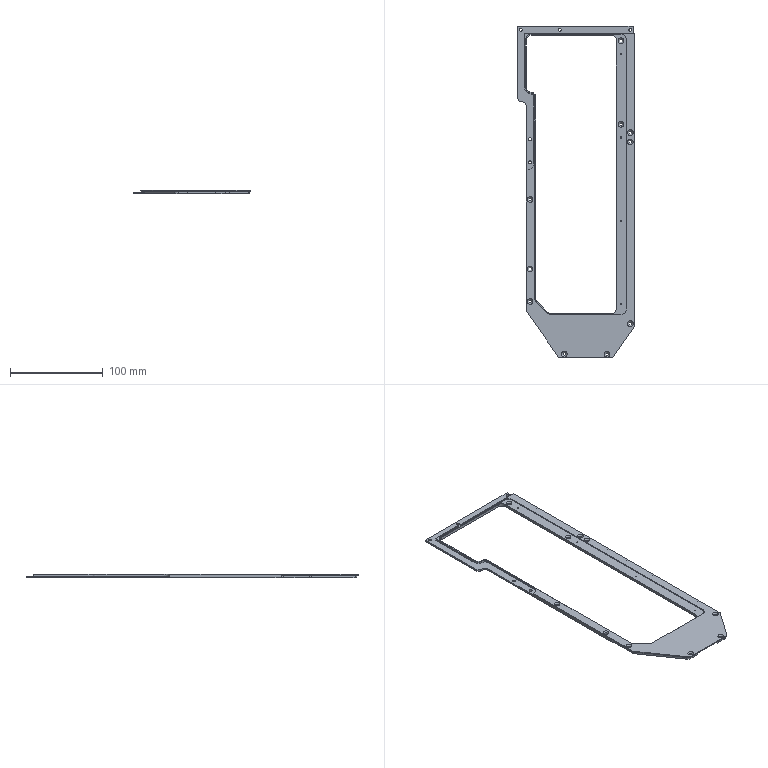CAM job | NX | 3-axis milling, drilling | part box 127 x 358 x 4 mm | stock box 134 x 366 x 4 mm
Tools:
number,name,description,diameter,corner_radius,flute_length,length,flutes
4,D6-18-D6-50-3T-ROUGH,D6-18-D6-50-3T-粗,6.0,0.0,18.0,50.0,2
5,D6-18-D6-50-3T-FINISH,D6-18-D6-50-3T,6.0,0.0,18.0,50.0,3
7,DRILL_D1.84-11-D3-40,钻刀D1.84-11-D3-40,1.84,0.0,11.0,12.0,2
3,DRILL_D3.2-42-71,钻刀D3.2-42-71,3.2,0.0,42.0,71.0,2
0,DRILL_D4.3-54-83,钻刀D4.3-54-83,4.3,0.0,54.0,83.0,2
2,DRILL_D5.3-62-92,钻刀D5.3-62-92,5.3,0.0,62.0,92.0,2
8,FORMTAP_M2-12-D3-39,挤压M2-12-D3-39,2.0,0.0,12.5,14.5,2
0,UPPERROW_M5-22-D5.5-60,上排M5-22-D5.5-60,5.0,0.0,22.0,25.0,2
6,CHAMFER_D3-90DEG,倒角D3-90度,3.0,0.0,5.0,50.0,2
1,CHAMFER_D8-90DEG,倒角D8-90度,8.0,0.0,8.0,60.0,2
Operations:
program,operation,operation_type,tool,method,geometry_group,spindle_rpm,surface_speed,feed_per_tooth,feed_cut,feed_plunge,cut_length_mm,path_length_mm,cut_time_min,machine_time_min
A1,SPOT_DRILL,Operation,CHAMFER_D8-90DEG,METHOD,WORKPIECE,2500.0,62.0,0.05,250.0,0.0,78.4,853.725,0.3136,0.3911
A1,SPOT_DRILL_COPY,Operation,DRILL_D5.3-62-92,METHOD,WORKPIECE,3000.0,0.0,0.0,200.0,0.0,133.0,962.925,0.665,0.748
A2,SPOT_DRILL_1,Operation,CHAMFER_D8-90DEG,METHOD,WORKPIECE,2500.0,62.0,0.05,250.0,0.0,69.0,907.539,0.276,0.3599
A2,SPOT_DRILL_1_COPY,Operation,DRILL_D3.2-42-71,METHOD,WORKPIECE,3000.0,0.0,0.0,200.0,0.0,135.0,1039.539,0.675,0.7655
A2,PLANAR_MILL_9,PlanarMilling,D6-18-D6-50-3T-ROUGH,METHOD,A-G54,3500.0,65.0,0.2143,1500.0,100.0,293.379,600.371,0.1956,0.2263
A2,FLOOR_FACING,VolumeBased25DMillingOperation,D6-18-D6-50-3T-ROUGH,METHOD,A-G54,3500.0,65.0,0.2143,1500.0,100.0,1620.379,1796.036,1.08,1.098
A2,PLANAR_MILL,PlanarMilling,D6-18-D6-50-3T-ROUGH,METHOD,A-G54,3500.0,65.0,0.2143,1500.0,100.0,168.708,207.508,0.1125,0.1164
A2,PLANAR_MILL_1_COPY_1,PlanarMilling,D6-18-D6-50-3T-ROUGH,METHOD,A-G54,3500.0,65.0,0.2143,1500.0,100.0,4139.758,4868.484,2.76,2.833
A2,PLANAR_MILL_1_COPY_1_COPY,PlanarMilling,D6-18-D6-50-3T-ROUGH,METHOD,A-G54,3500.0,65.0,0.2143,1500.0,100.0,715.0,1458.8,0.4767,0.551
A2,PLANAR_MILL_1,PlanarMilling,D6-18-D6-50-3T-ROUGH,METHOD,A-G54,3500.0,65.0,0.2143,1500.0,100.0,1614.092,2336.95,1.076,1.148
A2,PLANAR_MILL_9_COPY,PlanarMilling,D6-18-D6-50-3T-FINISH,METHOD,A-G54,3500.0,65.0,0.1429,500.0,100.0,80.291,394.36,0.1606,0.192
A2,FLOOR_FACING_COPY,VolumeBased25DMillingOperation,D6-18-D6-50-3T-FINISH,METHOD,A-G54,3500.0,65.0,0.0762,800.0,100.0,542.755,581.755,0.6784,0.6823
A2,PLANAR_MILL_COPY,PlanarMilling,D6-18-D6-50-3T-FINISH,METHOD,A-G54,3500.0,65.0,0.0762,800.0,100.0,169.908,208.908,0.2124,0.2163
A2,PLANAR_MILL_1_COPY_1_COPY_1,PlanarMilling,D6-18-D6-50-3T-FINISH,METHOD,A-G54,3500.0,65.0,0.0762,800.0,100.0,828.038,870.638,1.035,1.039
A2,PLANAR_MILL_1_COPY_1_COPY_COPY,PlanarMilling,D6-18-D6-50-3T-FINISH,METHOD,A-G54,3500.0,65.0,0.0762,800.0,100.0,143.4,186.0,0.1792,0.1835
A2,PLANAR_MILL_1_COPY,PlanarMilling,D6-18-D6-50-3T-FINISH,METHOD,A-G54,3500.0,65.0,0.0762,800.0,100.0,538.181,578.181,0.6727,0.6767
A3,PLANAR_MILL_7,PlanarMilling,CHAMFER_D3-90DEG,METHOD,A-G54,3000.0,28.0,0.1667,1000.0,100.0,1015.757,1050.957,1.016,1.019
A3,PLANAR_MILL_7_COPY,PlanarMilling,CHAMFER_D3-90DEG,METHOD,A-G54,3000.0,28.0,0.1667,1000.0,100.0,514.062,557.262,0.5141,0.5184
A3,PLANAR_MILL_7_COPY_COPY,PlanarMilling,CHAMFER_D3-90DEG,METHOD,A-G54,3000.0,28.0,0.1667,1000.0,100.0,68.503,362.572,0.0685,0.0979
B1,DRILLING,Operation,CHAMFER_D8-90DEG,METHOD,B-G55,2500.0,62.0,0.05,250.0,0.0,42.4,618.08,0.1696,0.2272
B1,PLANAR_MILL_2,PlanarMilling,D6-18-D6-50-3T-ROUGH,METHOD,B-G55,3500.0,65.0,0.1429,1000.0,100.0,1174.464,1911.807,1.175,1.248
B1,PLANAR_MILL_2_COPY,PlanarMilling,D6-18-D6-50-3T-ROUGH,METHOD,B-G55,3500.0,65.0,0.1429,1000.0,100.0,115.204,155.004,0.1152,0.1192
B1,PLANAR_MILL_3,PlanarMilling,D6-18-D6-50-3T-ROUGH,METHOD,B-G55,3500.0,65.0,0.1429,1000.0,100.0,793.361,829.161,0.7934,0.7969
B1,PLANAR_MILL_3_COPY,PlanarMilling,D6-18-D6-50-3T-ROUGH,METHOD,B-G55,3500.0,65.0,0.1429,1000.0,100.0,318.0,353.8,0.318,0.3216
B1,PLANAR_MILL_2_COPY_1,PlanarMilling,D6-18-D6-50-3T-FINISH,METHOD,B-G55,3500.0,65.0,0.0762,800.0,100.0,1176.104,1914.824,1.47,1.544
B1,PLANAR_MILL_2_COPY_COPY,PlanarMilling,D6-18-D6-50-3T-FINISH,METHOD,B-G55,3500.0,65.0,0.0762,800.0,100.0,119.204,159.203,0.149,0.153
B1,PLANAR_MILL_3_COPY_1_COPY,PlanarMilling,D6-18-D6-50-3T-FINISH,METHOD,B-G55,3500.0,65.0,0.0762,800.0,100.0,788.534,824.534,0.9857,0.9893
B1,PLANAR_MILL_3_COPY_1,PlanarMilling,D6-18-D6-50-3T-FINISH,METHOD,B-G55,3500.0,65.0,0.0762,800.0,100.0,793.989,829.989,0.9925,0.9961
B1,PLANAR_MILL_3_COPY_COPY,PlanarMilling,D6-18-D6-50-3T-FINISH,METHOD,B-G55,3500.0,65.0,0.0762,800.0,100.0,318.4,354.4,0.398,0.4016
B2,DRILLING_2,Operation,CHAMFER_D8-90DEG,METHOD,B-G55,2500.0,62.0,0.04,200.0,0.0,10.6,156.25,0.053,0.0676
B2,DRILLING_1,Operation,CHAMFER_D8-90DEG,METHOD,B-G55,2500.0,62.0,0.04,200.0,0.0,15.2,351.55,0.076,0.1096
B2,DRILLING_3,Operation,DRILL_D1.84-11-D3-40,METHOD,B-G55,1600.0,9.0,0.0312,100.0,0.0,32.0,385.15,0.32,0.3553
B3,PLANAR_MILL_5,PlanarMilling,CHAMFER_D3-90DEG,METHOD,B-G55,3000.0,28.0,0.1667,1000.0,100.0,921.602,959.602,0.9216,0.9254
B3,PLANAR_MILL_6,PlanarMilling,CHAMFER_D3-90DEG,METHOD,B-G55,3000.0,28.0,0.1667,1000.0,100.0,294.434,335.634,0.2944,0.2986
B3,PLANAR_MILL_5_COPY,PlanarMilling,CHAMFER_D3-90DEG,METHOD,B-G55,3000.0,28.0,0.1667,1000.0,100.0,804.725,841.925,0.8047,0.8084
B6,DRILLING_3_COPY,Operation,FORMTAP_M2-12-D3-39,METHOD,B-G55,300.0,1.0,0.2,120.0,0.0,30.0,381.15,0.25,0.2851
B6,PLANAR_MILL_4,PlanarMilling,D6-18-D6-50-3T-ROUGH,METHOD,B-G55,3500.0,65.0,0.2143,1500.0,100.0,8012.729,8057.029,5.342,5.346
B6,PLANAR_MILL_4_COPY,PlanarMilling,D6-18-D6-50-3T-FINISH,METHOD,B-G55,3500.0,65.0,0.0762,800.0,100.0,1525.011,1569.611,1.906,1.911
B6,PLANAR_MILL_5_COPY_COPY,PlanarMilling,CHAMFER_D3-90DEG,METHOD,B-G55,3000.0,28.0,0.1667,1000.0,100.0,778.077,817.277,0.7781,0.782
NC_PROGRAM,SPOT_DRILL_COPY_1_COPY,Operation,CHAMFER_D8-90DEG,METHOD,C-G56,2500.0,62.0,0.05,250.0,0.0,11.2,81.498,0.0448,0.0518
NC_PROGRAM,SPOT_DRILL_COPY_COPY_COPY_1,Operation,DRILL_D4.3-54-83,METHOD,C-G56,3000.0,0.0,0.0,200.0,0.0,36.0,131.098,0.18,0.1895
FIXTURE_1,SPOT_DRILL_COPY_1,Operation,CHAMFER_D8-90DEG,METHOD,WORKPIECE,2500.0,62.0,0.05,250.0,0.0,67.2,798.835,0.2688,0.342
FIXTURE_1,PLANAR_MILL_8,PlanarMilling,CHAMFER_D8-90DEG,METHOD,A-G54,3000.0,75.0,0.1667,1000.0,100.0,522.0,556.2,0.522,0.5254
FIXTURE_1,SPOT_DRILL_COPY_COPY,Operation,DRILL_D4.3-54-83,METHOD,WORKPIECE,3000.0,0.0,0.0,200.0,0.0,216.0,1096.435,1.08,1.168
FIXTURE_1,SPOT_DRILL_COPY_COPY_COPY,Operation,UPPERROW_M5-22-D5.5-60,METHOD,WORKPIECE,300.0,3.0,0.4,240.0,0.0,156.0,976.435,0.65,0.732